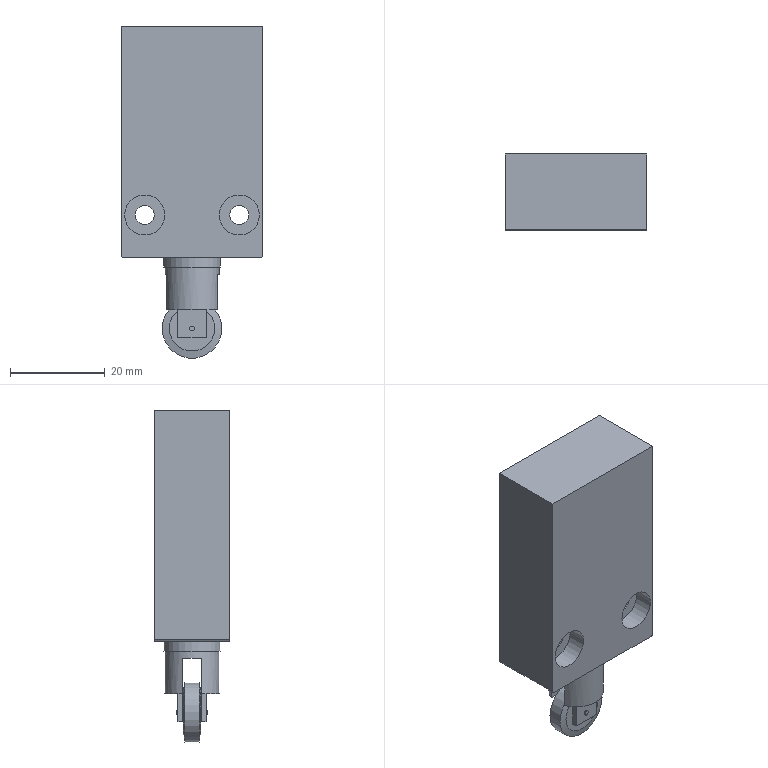Part | STEP file | solid 163 | 1 solid | 45 faces | box 30 x 16 x 70.3 mm | volume 23738 mm3 | plane 28 | cylinder 15 | cone 2 | commonest cylinder face diameters 1 x6 8.5 x4 4 x2 11.5 x1 12 x1 12.6 x1